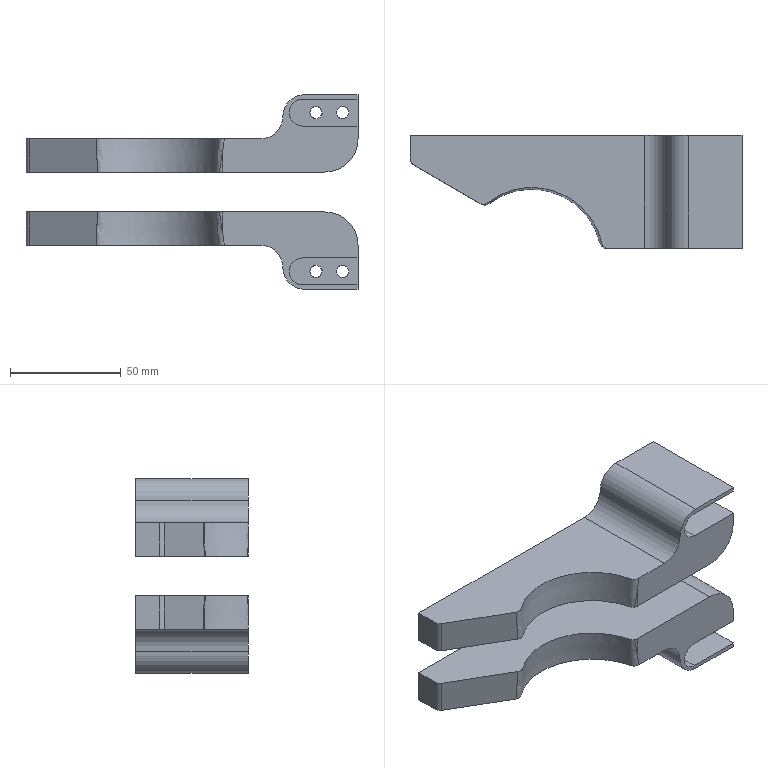NC program | NX | posted with a generic post | part box 150 x 51 x 88 mm
Lines 9175 to 9990 of 21241:
(FIXED_CONTOUR , TOOL : R4)
N18306 T08 M6
N18308 G54
N18310 G17 G0 G90 X12.055 Y-18.193 S9500 M3
N18312 G43 Z30. H8
N18314 Z4.4
N18316 G94 G1 Z0.185 F3000.
N18318 Y-18.066 Z0.019
N18320 Y-17.9 Z-0.108
N18322 Y-17.707 Z-0.188
N18324 Y-17.5 Z-0.215
N18326 X12.054 Y-13.737 Z-0.213
N18328 X12.065 Y-11.855 Z-0.236
N18330 X12.08 Y-9.973 Z-0.27
N18332 X12.09 Y-9.033 Z-0.29
N18334 X12.106 Y-8.383 Z-0.302
N18336 X12.156 Y-7.908 Z-0.298
N18338 X12.376 Y-6.012 Z-0.279
N18340 X12.618 Y-4.124 Z-0.251
N18342 X12.746 Y-3.183 Z-0.234
N18344 X12.88 Y-2.245 Z-0.219
N18346 X12.781 Y-2.244 Z-0.244
N18348 X12.649 Y-3.183 Z-0.261
N18350 X12.522 Y-4.124 Z-0.279
N18352 X12.28 Y-6.011 Z-0.308
N18354 X12.061 Y-7.907 Z-0.329
N18356 X12.011 Y-8.383 Z-0.333
N18358 X11.995 Y-9.033 Z-0.321
N18360 X11.985 Y-9.973 Z-0.301
N18362 X11.957 Y-13.737 Z-0.239
N18364 X11.958 Y-17.5 Z-0.24
N18366 X11.861 Z-0.267
N18368 Y-13.737
N18370 X11.89 Y-9.974 Z-0.332
N18372 X11.9 Y-9.033 Z-0.353
N18374 X11.917 Y-8.383 Z-0.365
N18376 X11.967 Y-7.907 Z-0.361
N18378 X12.185 Y-6.011 Z-0.339
N18380 X12.425 Y-4.123 Z-0.308
N18382 X12.552 Y-3.182 Z-0.289
N18384 X12.684 Y-2.243 Z-0.271
N18386 X12.587 Z-0.299
N18388 X12.456 Y-3.182 Z-0.318
N18390 X12.329 Y-4.123 Z-0.338
N18392 X12.09 Y-6.011 Z-0.371
N18394 X11.873 Y-7.907 Z-0.395
N18396 X11.823 Y-8.383 Z-0.399
N18398 X11.806 Y-9.033 Z-0.387
N18400 X11.796 Y-9.974 Z-0.365
N18402 X11.766 Y-13.737 Z-0.297
N18404 X11.765 Y-17.5 Z-0.295
N18406 X11.669 Z-0.325
N18408 X11.671 Y-13.737 Z-0.33
N18410 X11.703 Y-9.974 Z-0.399
N18412 X11.713 Y-9.033 Z-0.422
N18414 X11.73 Y-8.383 Z-0.434
N18416 X11.78 Y-7.907 Z-0.429
N18418 X11.996 Y-6.011 Z-0.405
N18420 X12.234 Y-4.122 Z-0.37
N18422 X12.36 Y-3.181 Z-0.349
N18424 X12.491 Y-2.242 Z-0.329
N18426 X12.395 Z-0.36
N18428 X12.265 Y-3.181 Z-0.381
N18430 X12.14 Y-4.122 Z-0.403
N18432 X11.902 Y-6.01 Z-0.439
N18434 X11.687 Y-7.907 Z-0.465
N18436 X11.638 Y-8.383 Z-0.471
N18438 X11.62 Y-9.033 Z-0.458
N18440 X11.61 Y-9.974 Z-0.435
N18442 X11.578 Y-13.737 Z-0.365
N18444 X11.574 Y-17.5 Z-0.355
N18446 X11.479 Z-0.387
N18448 X11.485 Y-13.737 Z-0.399
N18450 X11.518 Y-9.974 Z-0.471
N18452 X11.528 Y-9.033 Z-0.495
N18454 X11.546 Y-8.383 Z-0.508
N18456 X11.595 Y-7.907 Z-0.503
N18458 X11.809 Y-6.01 Z-0.475
N18460 X12.046 Y-4.122 Z-0.437
N18462 X12.17 Y-3.181 Z-0.414
N18464 X12.3 Y-2.241 Z-0.392
N18466 X12.205 Z-0.425
N18468 X12.076 Y-3.18 Z-0.449
N18470 X11.952 Y-4.122 Z-0.473
N18472 X11.717 Y-6.01 Z-0.513
N18474 X11.503 Y-7.907 Z-0.541
N18476 X11.454 Y-8.383 Z-0.547
N18478 X11.437 Y-9.033 Z-0.534
N18480 X11.426 Y-9.974 Z-0.509
N18482 X11.392 Y-13.737 Z-0.435
N18484 X11.386 Y-17.5 Z-0.421
N18486 X11.292 Z-0.455
N18488 Y-15.618
N18490 X11.3 Y-13.737 Z-0.471
N18492 X11.335 Y-9.974 Z-0.549
N18494 X11.346 Y-9.033 Z-0.574
N18496 X11.364 Y-8.383 Z-0.587
N18498 X11.412 Y-7.907 Z-0.581
N18500 X11.625 Y-6.01 Z-0.551
N18502 X11.859 Y-4.122 Z-0.51
N18504 X11.983 Y-3.18 Z-0.484
N18506 X12.111 Y-2.241 Z-0.46
N18508 X12.017 Z-0.496
N18510 X11.89 Y-3.18 Z-0.522
N18512 X11.767 Y-4.122 Z-0.548
N18514 X11.534 Y-6.011 Z-0.591
N18516 X11.322 Y-7.907 Z-0.622
N18518 X11.273 Y-8.383 Z-0.629
N18520 X11.256 Y-9.033 Z-0.615
N18522 X11.244 Y-9.974 Z-0.589
N18524 X11.208 Y-13.737 Z-0.51
N18526 X11.199 Y-15.618 Z-0.491
N18528 X11.2 Y-17.5
N18530 X11.107 Z-0.528
N18532 Y-15.618
N18534 X11.117 Y-13.737 Z-0.549
N18536 X11.154 Y-9.974 Z-0.631
N18538 X11.166 Y-9.033 Z-0.657
N18540 X11.184 Y-8.383 Z-0.671
N18542 X11.232 Y-7.908 Z-0.665
N18544 X11.443 Y-6.011 Z-0.632
N18546 X11.676 Y-4.122 Z-0.587
N18548 X11.798 Y-3.181 Z-0.56
N18550 X11.925 Y-2.241 Z-0.533
N18552 X11.832 Z-0.572
N18554 X11.706 Y-3.181 Z-0.6
N18556 X11.585 Y-4.122 Z-0.628
N18558 X11.353 Y-6.011 Z-0.674
N18560 X11.143 Y-7.908 Z-0.709
N18562 X11.095 Y-8.384 Z-0.715
N18564 X11.077 Y-9.033 Z-0.701
N18566 X11.065 Y-9.974 Z-0.674
N18568 X11.026 Y-13.737 Z-0.59
N18570 X11.016 Y-15.618 Z-0.568
N18572 Y-17.5 Z-0.567
N18574 X10.925 Z-0.607
N18576 X10.926 Y-15.618 Z-0.61
N18578 X10.937 Y-13.737 Z-0.632
N18580 X10.976 Y-9.974 Z-0.719
N18582 X10.988 Y-9.033 Z-0.746
N18584 X11.006 Y-8.384 Z-0.761
N18586 X11.054 Y-7.909 Z-0.754
N18588 X11.264 Y-6.012 Z-0.718
N18590 X11.494 Y-4.123 Z-0.67
N18592 X11.615 Y-3.181 Z-0.641
N18594 X11.741 Y-2.241 Z-0.612
N18596 X11.65 Y-2.242 Z-0.653
N18598 X11.525 Y-3.181 Z-0.683
N18600 X11.404 Y-4.123 Z-0.713
N18602 X11.175 Y-6.012 Z-0.763
N18604 X10.966 Y-7.909 Z-0.8
N18606 X10.918 Y-8.385 Z-0.807
N18608 X10.9 Y-9.033 Z-0.792
N18610 X10.888 Y-9.974 Z-0.764
N18612 X10.847 Y-13.737 Z-0.675
N18614 X10.837 Y-15.618 Z-0.652
N18616 X10.835 Y-17.5 Z-0.648
N18618 X10.745 Z-0.69
N18620 X10.747 Y-15.618 Z-0.695
N18622 X10.758 Y-13.737 Z-0.72
N18624 X10.8 Y-9.974 Z-0.811
N18626 X10.813 Y-9.033 Z-0.84
N18628 X10.831 Y-8.385 Z-0.855
N18630 X10.879 Y-7.91 Z-0.848
N18632 X11.086 Y-6.013 Z-0.809
N18634 X11.315 Y-4.124 Z-0.758
N18636 X11.559 Y-2.242 Z-0.696
N18638 X11.469 Z-0.74
N18640 X11.226 Y-4.124 Z-0.804
N18642 X10.999 Y-6.013 Z-0.857
N18644 X10.792 Y-7.91 Z-0.896
N18646 X10.744 Y-8.386 Z-0.904
N18648 X10.726 Y-9.033 Z-0.889
N18650 X10.713 Y-9.974 Z-0.859
N18652 X10.67 Y-13.737 Z-0.766
N18654 X10.659 Y-15.618 Z-0.74
N18656 X10.656 Y-17.5 Z-0.734
N18658 X10.567 Z-0.779
N18660 X10.57 Y-15.618 Z-0.786
N18662 X10.583 Y-13.737 Z-0.813
N18664 X10.626 Y-9.974 Z-0.909
N18666 X10.64 Y-9.033 Z-0.939
N18668 X10.658 Y-8.386 Z-0.955
N18670 X10.706 Y-7.911 Z-0.947
N18672 X10.912 Y-6.014 Z-0.906
N18674 X11.138 Y-4.125 Z-0.851
N18676 X11.38 Y-2.243 Z-0.785
N18678 X11.291 Y-2.244 Z-0.832
N18680 X11.051 Y-4.125 Z-0.9
N18682 X10.825 Y-6.015 Z-0.956
N18684 X10.62 Y-7.912 Z-0.998
N18686 X10.573 Y-8.387 Z-1.006
N18688 X10.554 Y-9.033 Z-0.99
N18690 X10.54 Y-9.974 Z-0.96
N18692 X10.496 Y-13.737 Z-0.861
N18694 X10.483 Y-15.618 Z-0.833
N18696 X10.479 Y-17.5 Z-0.825
N18698 X10.392 Z-0.872
N18700 X10.396 Y-15.618 Z-0.882
N18702 X10.409 Y-13.737 Z-0.911
N18704 X10.455 Y-9.974 Z-1.012
N18706 X10.469 Y-9.033 Z-1.043
N18708 X10.488 Y-8.388 Z-1.06
N18710 X10.535 Y-7.912 Z-1.051
N18712 X10.739 Y-6.016 Z-1.007
N18714 X10.964 Y-4.126 Z-0.949
N18716 X11.203 Y-2.244 Z-0.879
N18718 X11.116 Y-2.245 Z-0.928
N18720 X10.877 Y-4.127 Z-1.
N18722 X10.654 Y-6.016 Z-1.06
N18724 X10.45 Y-7.913 Z-1.105
N18726 X10.404 Y-8.389 Z-1.114
N18728 X10.385 Y-9.033 Z-1.097
N18730 X10.37 Y-9.974 Z-1.065
N18732 X10.323 Y-13.737 Z-0.962
N18734 X10.31 Y-15.618 Z-0.932
N18736 X10.305 Y-17.5 Z-0.921
N18738 X10.218 Z-0.971
N18740 X10.224 Y-15.619 Z-0.983
N18742 X10.238 Y-13.737 Z-1.015
N18744 X10.286 Y-9.974 Z-1.12
N18746 X10.301 Y-9.033 Z-1.153
N18748 X10.32 Y-8.39 Z-1.17
N18750 X10.367 Y-7.914 Z-1.16
N18752 X10.569 Y-6.017 Z-1.114
N18754 X10.791 Y-4.128 Z-1.053
N18756 X11.029 Y-2.246 Z-0.979
N18758 X10.942 Y-2.247 Z-1.031
N18760 X10.706 Y-4.129 Z-1.107
N18762 X10.485 Y-6.018 Z-1.169
N18764 X10.283 Y-7.915 Z-1.217
N18766 X10.237 Y-8.391 Z-1.227
N18768 X10.218 Y-9.033 Z-1.209
N18770 X10.203 Y-9.974 Z-1.176
N18772 X10.154 Y-13.737 Z-1.068
N18774 X10.139 Y-15.619 Z-1.036
N18776 X10.133 Y-17.5 Z-1.023
N18778 X10.048 Z-1.075
N18780 X10.054 Y-15.619 Z-1.089
N18782 X10.07 Y-13.737 Z-1.123
N18784 X10.12 Y-9.974 Z-1.234
N18786 X10.135 Y-9.033 Z-1.267
N18788 X10.154 Y-8.392 Z-1.285
N18790 X10.201 Y-7.916 Z-1.275
N18792 X10.401 Y-6.02 Z-1.226
N18794 X10.622 Y-4.13 Z-1.162
N18796 X10.856 Y-2.248 Z-1.084
N18798 X10.771 Y-2.249 Z-1.138
N18800 X10.538 Y-4.132 Z-1.218
N18802 X10.318 Y-6.021 Z-1.284
N18804 X10.119 Y-7.917 Z-1.335
N18806 X10.072 Y-8.393 Z-1.345
N18808 X10.053 Y-9.033 Z-1.327
N18810 X10.038 Y-9.974 Z-1.293
N18812 X9.986 Y-13.737 Z-1.18
N18814 X9.97 Y-15.619 Z-1.145
N18816 X9.963 Y-17.5 Z-1.129
N18818 X9.879 Z-1.184
N18820 X9.887 Y-15.619 Z-1.201
N18822 X9.903 Y-13.737 Z-1.237
N18824 X9.956 Y-9.974 Z-1.353
N18826 X9.972 Y-9.033 Z-1.388
N18828 X9.991 Y-8.394 Z-1.406
N18830 X10.037 Y-7.919 Z-1.395
N18832 X10.236 Y-6.022 Z-1.344
N18834 X10.454 Y-4.133 Z-1.276
N18836 X10.687 Y-2.25 Z-1.194
N18838 X10.603 Y-2.252 Z-1.251
N18840 X10.372 Y-4.134 Z-1.335
N18842 X10.154 Y-6.023 Z-1.405
N18844 X9.956 Y-7.92 Z-1.458
N18846 X9.91 Y-8.395 Z-1.468
N18848 X9.891 Y-9.033 Z-1.45
N18850 X9.875 Y-9.974 Z-1.414
N18852 X9.821 Y-13.737 Z-1.296
N18854 X9.804 Y-15.619 Z-1.259
N18856 X9.796 Y-17.5 Z-1.241
N18858 X9.713 Z-1.299
N18860 X9.722 Y-15.619 Z-1.318
N18862 X9.74 Y-13.737 Z-1.357
N18864 X9.794 Y-9.974 Z-1.477
N18866 X9.811 Y-9.033 Z-1.513
N18868 X9.83 Y-8.396 Z-1.532
N18870 X9.876 Y-7.921 Z-1.521
N18872 X10.073 Y-6.025 Z-1.467
N18874 X10.29 Y-4.136 Z-1.396
N18876 X10.519 Y-2.253 Z-1.31
N18878 X10.437 Y-2.255 Z-1.369
N18880 X10.208 Y-4.137 Z-1.458
N18882 X9.993 Y-6.026 Z-1.53
N18884 X9.796 Y-7.923 Z-1.586
N18886 X9.751 Y-8.398 Z-1.597
N18888 X9.731 Y-9.033 Z-1.578
N18890 X9.715 Y-9.974 Z-1.542
N18892 X9.659 Y-13.737 Z-1.418
N18894 X9.64 Y-15.619 Z-1.379
N18896 X9.631 Y-17.5 Z-1.359
N18898 X9.55 Z-1.419
N18900 X9.56 Y-15.619 Z-1.44
N18902 X9.578 Y-13.737 Z-1.482
N18904 X9.635 Y-9.974 Z-1.607
N18906 X9.653 Y-9.034 Z-1.645
N18908 X9.672 Y-8.399 Z-1.664
N18910 X9.718 Y-7.924 Z-1.653
N18912 X9.913 Y-6.028 Z-1.595
N18914 X10.127 Y-4.139 Z-1.521
N18916 X10.355 Y-2.256 Z-1.431
N18918 X10.273 Y-2.258 Z-1.493
N18920 X10.047 Y-4.14 Z-1.586
N18922 X9.834 Y-6.03 Z-1.662
N18924 X9.639 Y-7.926 Z-1.72
N18926 X9.594 Y-8.401 Z-1.732
N18928 X9.574 Y-9.034 Z-1.713
N18930 X9.557 Y-9.974 Z-1.675
N18932 X9.499 Y-13.737 Z-1.546
N18934 X9.479 Y-15.619 Z-1.504
N18936 X9.469 Y-17.5 Z-1.481
N18938 X9.389 Z-1.545
N18940 X9.4 Y-15.619 Z-1.568
N18942 X9.42 Y-13.737 Z-1.612
N18944 X9.479 Y-9.974 Z-1.743
N18946 X9.497 Y-9.034 Z-1.782
N18948 X9.517 Y-8.402 Z-1.802
N18950 X9.562 Y-7.927 Z-1.79
N18952 X9.755 Y-6.031 Z-1.73
N18954 X9.967 Y-4.142 Z-1.652
N18956 X10.192 Y-2.26 Z-1.557
N18958 X10.112 Y-2.261 Z-1.623
N18960 X9.889 Y-4.144 Z-1.719
N18962 X9.678 Y-6.033 Z-1.799
N18964 X9.485 Y-7.929 Z-1.86
N18966 X9.44 Y-8.404 Z-1.873
N18968 X9.42 Y-9.034 Z-1.853
N18970 X9.402 Y-9.974 Z-1.813
N18972 X9.341 Y-13.737 Z-1.679
N18974 X9.321 Y-15.619 Z-1.635
N18976 X9.31 Y-17.5 Z-1.61
N18978 X9.231 Z-1.676
N18980 X9.242 Y-15.619 Z-1.702
N18982 X9.263 Y-13.737 Z-1.748
N18984 X9.326 Y-9.974 Z-1.885
N18986 X9.344 Y-9.034 Z-1.925
N18988 X9.364 Y-8.406 Z-1.945
N18990 X9.409 Y-7.931 Z-1.933
N18992 X9.6 Y-6.035 Z-1.87
N18994 X9.81 Y-4.146 Z-1.788
N18996 X10.033 Y-2.263 Z-1.69
N18998 X9.954 Y-2.265 Z-1.758
N19000 X9.733 Y-4.148 Z-1.859
N19002 X9.524 Y-6.037 Z-1.942
N19004 X9.333 Y-7.932 Z-2.007
N19006 X9.289 Y-8.407 Z-2.02
N19008 X9.268 Y-9.034 Z-1.999
N19010 X9.25 Y-9.974 Z-1.958
N19012 X9.186 Y-13.737 Z-1.819
N19014 X9.165 Y-15.619 Z-1.771
N19016 X9.152 Y-17.5 Z-1.744
N19018 X9.075 Z-1.813
N19020 X9.088 Y-15.619 Z-1.842
N19022 X9.11 Y-13.737 Z-1.89
N19024 X9.175 Y-9.974 Z-2.033
N19026 X9.194 Y-9.034 Z-2.074
N19028 X9.214 Y-8.409 Z-2.095
N19030 X9.258 Y-7.934 Z-2.082
N19032 X9.448 Y-6.039 Z-2.016
N19034 X9.656 Y-4.15 Z-1.931
N19036 X9.876 Y-2.268 Z-1.828
N19038 X9.798 Y-2.27 Z-1.9
N19040 X9.58 Y-4.153 Z-2.005
N19042 X9.373 Y-6.041 Z-2.092
N19044 X9.184 Y-7.936 Z-2.159
N19046 X9.14 Y-8.411 Z-2.172
N19048 X9.12 Y-9.034 Z-2.151
N19050 X9.1 Y-9.974 Z-2.109
N19052 X9.034 Y-13.737 Z-1.964
N19054 X9.011 Y-15.619 Z-1.914
N19056 X8.998 Y-17.5 Z-1.884
N19058 X8.922 Z-1.956
N19060 X8.936 Y-15.619 Z-1.987
N19062 X8.959 Y-13.737 Z-2.039
N19064 X9.027 Y-9.974 Z-2.187
N19066 X9.046 Y-9.034 Z-2.23
N19068 X9.067 Y-8.413 Z-2.251
N19070 X9.111 Y-7.938 Z-2.237
N19072 X9.299 Y-6.043 Z-2.169
N19074 X9.504 Y-4.155 Z-2.08
N19076 X9.721 Y-2.272 Z-1.973
N19078 X9.645 Y-2.275 Z-2.047
N19080 X9.429 Y-4.157 Z-2.157
N19082 X9.225 Y-6.046 Z-2.247
N19084 X9.038 Y-7.94 Z-2.318
N19086 X8.994 Y-8.415 Z-2.332
N19088 X8.974 Y-9.034 Z-2.31
N19090 X8.954 Y-9.974 Z-2.266
N19092 X8.885 Y-13.737 Z-2.115
N19094 X8.861 Y-15.619 Z-2.062
N19096 X8.846 Y-17.5 Z-2.03
N19098 X8.772 Z-2.105
N19100 X8.787 Y-15.619 Z-2.139
N19102 X8.812 Y-13.737 Z-2.193
N19104 X8.882 Y-9.974 Z-2.347
N19106 X8.902 Y-9.034 Z-2.392
N19108 X8.923 Y-8.417 Z-2.414
N19110 X8.966 Y-7.942 Z-2.399
N19112 X9.152 Y-6.048 Z-2.328
N19114 X9.355 Y-4.16 Z-2.235
N19116 X9.57 Y-2.277 Z-2.123
N19118 X9.495 Y-2.28 Z-2.201
N19120 X9.282 Y-4.162 Z-2.315
N19122 X9.08 Y-6.051 Z-2.41
N19124 X8.895 Y-7.945 Z-2.483
N19126 X8.852 Y-8.419 Z-2.498
N19128 X8.831 Y-9.034 Z-2.476
N19130 X8.81 Y-9.975 Z-2.43
N19132 X8.739 Y-13.737 Z-2.273
N19134 X8.713 Y-15.619 Z-2.217
N19136 X8.697 Y-17.5 Z-2.182
N19138 X8.624 Z-2.261
N19140 X8.641 Y-15.619 Z-2.297
N19142 X8.667 Y-13.737 Z-2.354
N19144 X8.74 Y-9.975 Z-2.515
N19146 X8.761 Y-9.034 Z-2.561
N19148 X8.782 Y-8.422 Z-2.583
N19150 X8.825 Y-7.947 Z-2.568
N19152 X9.009 Y-6.053 Z-2.493
N19154 X9.209 Y-4.165 Z-2.397
N19156 X9.421 Y-2.282 Z-2.28
N19158 X9.348 Y-2.285 Z-2.362
N19160 X9.138 Y-4.168 Z-2.48
N19162 X8.938 Y-6.056 Z-2.579
N19164 X8.755 Y-7.949 Z-2.655
N19166 X8.712 Y-8.424 Z-2.671
N19168 X8.691 Y-9.034 Z-2.648
N19170 X8.67 Y-9.975 Z-2.601
N19172 X8.595 Y-13.737 Z-2.437
N19174 X8.569 Y-15.619 Z-2.378
N19176 X8.552 Y-17.5 Z-2.341
N19178 X8.48 Z-2.423
N19180 X8.497 Y-15.619 Z-2.462
N19182 X8.525 Y-13.737 Z-2.522
N19184 X8.601 Y-9.975 Z-2.689
N19186 X8.623 Y-9.034 Z-2.737
N19188 X8.644 Y-8.426 Z-2.76
N19190 X8.686 Y-7.952 Z-2.744
N19192 X8.868 Y-6.059 Z-2.666
N19194 X9.067 Y-4.171 Z-2.565
N19196 X9.276 Y-2.288 Z-2.444
N19198 X9.204 Y-2.291 Z-2.529
N19200 X8.996 Y-4.174 Z-2.652
N19202 X8.8 Y-6.061 Z-2.755
N19204 X8.619 Y-7.955 Z-2.835
N19206 X8.576 Y-8.429 Z-2.851
N19208 X8.555 Y-9.034 Z-2.828
N19210 X8.533 Y-9.975 Z-2.779
N19212 X8.455 Y-13.737 Z-2.609
N19214 X8.427 Y-15.619 Z-2.547
N19216 X8.409 Y-17.5 Z-2.506
N19218 X8.338 Z-2.591
N19220 X8.357 Y-15.619 Z-2.633
N19222 X8.386 Y-13.737 Z-2.697
N19224 X8.465 Y-9.975 Z-2.871
N19226 X8.488 Y-9.034 Z-2.921
N19228 X8.51 Y-8.431 Z-2.944
N19230 X8.552 Y-7.957 Z-2.928
N19232 X8.732 Y-6.064 Z-2.846
N19234 X8.927 Y-4.177 Z-2.741
N19236 X9.133 Y-2.294 Z-2.615
N19238 X9.063 Y-2.298 Z-2.703
N19240 X8.859 Y-4.18 Z-2.832
N19242 X8.664 Y-6.067 Z-2.939
N19244 X8.486 Y-7.96 Z-3.022
N19246 X8.444 Y-8.434 Z-3.039
N19248 X8.422 Y-9.034 Z-3.016
N19250 X8.399 Y-9.975 Z-2.965
N19252 X8.318 Y-13.737 Z-2.787
N19254 X8.289 Y-15.619 Z-2.722
N19256 X8.269 Y-17.5 Z-2.678
N19258 X8.2 Z-2.767
N19260 X8.221 Y-15.619 Z-2.812
N19262 X8.251 Y-13.737 Z-2.88
N19264 X8.334 Y-9.975 Z-3.061
N19266 X8.357 Y-9.034 Z-3.113
N19268 X8.379 Y-8.437 Z-3.137
N19270 X8.42 Y-7.963 Z-3.119
N19272 X8.598 Y-6.071 Z-3.033
N19274 X8.791 Y-4.183 Z-2.924
N19276 X8.994 Y-2.301 Z-2.793
N19278 X8.926 Y-2.304 Z-2.885
N19280 X8.724 Y-4.187 Z-3.019
N19282 X8.533 Y-6.074 Z-3.13
N19284 X8.356 Y-7.966 Z-3.218
N19286 X8.315 Y-8.44 Z-3.236
N19288 X8.293 Y-9.034 Z-3.212
N19290 X8.269 Y-9.975 Z-3.159
N19292 X8.185 Y-13.737 Z-2.974
N19294 X8.154 Y-15.619 Z-2.905
N19296 X8.133 Y-17.5 Z-2.858
N19298 X8.066 Z-2.951
N19300 X8.088 Y-15.619 Z-2.999
N19302 X8.12 Y-13.737 Z-3.07
N19304 X8.206 Y-9.975 Z-3.259
N19306 X8.23 Y-9.034 Z-3.313
N19308 X8.252 Y-8.443 Z-3.337
N19310 X8.293 Y-7.969 Z-3.319
N19312 X8.468 Y-6.077 Z-3.229
N19314 X8.658 Y-4.19 Z-3.115
N19316 X8.859 Y-2.308 Z-2.979
N19318 X8.792 Y-2.312 Z-3.075
N19320 X8.594 Y-4.194 Z-3.214
N19322 X8.405 Y-6.081 Z-3.331
N19324 X8.231 Y-7.972 Z-3.422
N19326 X8.19 Y-8.446 Z-3.441
N19328 X8.168 Y-9.034 Z-3.416
N19330 X8.143 Y-9.975 Z-3.361
N19332 X8.055 Y-13.737 Z-3.168
N19334 X8.022 Y-15.619 Z-3.096
N19336 X8. Y-17.5 Z-3.046
N19338 X7.935 Z-3.142
N19340 X7.958 Y-15.619 Z-3.194
N19342 X7.992 Y-13.737 Z-3.269
N19344 X8.082 Y-9.975 Z-3.466
N19346 X8.107 Y-9.034 Z-3.522
N19348 X8.129 Y-8.449 Z-3.547
N19350 X8.17 Y-7.975 Z-3.528
N19352 X8.343 Y-6.084 Z-3.434
N19354 X8.53 Y-4.198 Z-3.315
N19356 X8.727 Y-2.316 Z-3.173
N19358 X8.662 Y-2.32 Z-3.273
N19360 X8.467 Y-4.202 Z-3.418
N19362 X8.281 Y-6.088 Z-3.54
N19364 X8.11 Y-7.979 Z-3.636
N19366 X8.07 Y-8.452 Z-3.655
N19368 X8.047 Y-9.034 Z-3.63
N19370 X8.021 Y-9.975 Z-3.573
N19372 X7.93 Y-13.737 Z-3.371
N19374 X7.895 Y-15.619 Z-3.295
N19376 X7.871 Y-17.5 Z-3.241
N19378 X7.807 Z-3.342
N19380 X7.833 Y-15.619 Z-3.398
N19382 X7.868 Y-13.737 Z-3.476
N19384 X7.962 Y-9.975 Z-3.682
N19386 X7.989 Y-9.034 Z-3.741
N19388 X8.011 Y-8.455 Z-3.766
N19390 X8.051 Y-7.982 Z-3.746
N19392 X8.221 Y-6.092 Z-3.648
N19394 X8.405 Y-4.206 Z-3.524
N19396 X8.599 Y-2.324 Z-3.376
N19398 X8.536 Y-2.328 Z-3.481
N19400 X8.344 Y-4.21 Z-3.632
N19402 X8.162 Y-6.096 Z-3.759
N19404 X7.993 Y-7.986 Z-3.859
N19406 X7.954 Y-8.459 Z-3.88
N19408 X7.931 Y-9.034 Z-3.854
N19410 X7.904 Y-9.975 Z-3.794
N19412 X7.808 Y-13.737 Z-3.584
N19414 X7.771 Y-15.619 Z-3.503
N19416 X7.745 Y-17.5 Z-3.445
N19418 X7.715 Z-3.498
N19420 X7.684 Z-3.551
N19422 X7.711 Y-15.619 Z-3.61
N19424 X7.749 Y-13.737 Z-3.693
N19426 X7.847 Y-9.975 Z-3.909
N19428 X7.875 Y-9.034 Z-3.97
N19430 X7.898 Y-8.463 Z-3.996
N19432 X7.937 Y-7.99 Z-3.975
N19434 X8.104 Y-6.1 Z-3.872
N19436 X8.285 Y-4.214 Z-3.742
N19438 X8.475 Y-2.332 Z-3.588
N19440 X8.445 Y-2.335 Z-3.643
N19442 X8.415 Y-2.337 Z-3.698
N19444 X8.227 Y-4.219 Z-3.855
N19446 X8.047 Y-6.104 Z-3.988
N19448 X7.882 Y-7.993 Z-4.094
N19450 X7.843 Y-8.466 Z-4.116
N19452 X7.82 Y-9.034 Z-4.089
N19454 X7.791 Y-9.975 Z-4.027
N19456 X7.691 Y-13.737 Z-3.806
N19458 X7.652 Y-15.619 Z-3.721
N19460 X7.624 Y-17.5 Z-3.659
N19462 X7.595 Z-3.714
N19464 X7.566 Z-3.77
N19466 X7.595 Y-15.619 Z-3.833
N19468 X7.634 Y-13.737 Z-3.921
N19470 X7.737 Y-9.975 Z-4.147
N19472 X7.766 Y-9.034 Z-4.211
N19474 X7.789 Y-8.47 Z-4.238
N19476 X7.828 Y-7.997 Z-4.216
N19478 X7.992 Y-6.109 Z-4.107
N19480 X8.169 Y-4.224 Z-3.971
N19482 X8.355 Y-2.342 Z-3.81
N19484 X8.326 Y-2.344 Z-3.867
N19486 X8.298 Y-2.346 Z-3.925
N19488 X8.114 Y-4.228 Z-4.09
N19490 X7.938 Y-6.113 Z-4.229
N19492 X7.775 Y-8.001 Z-4.341
N19494 X7.737 Y-8.474 Z-4.363
N19496 X7.714 Y-9.034 Z-4.336
N19498 X7.684 Y-9.975 Z-4.271
N19500 X7.579 Y-13.738 Z-4.039
N19502 X7.538 Y-15.619 Z-3.949
N19504 X7.521 Y-16.559 Z-3.912
N19506 X7.508 Y-17.5 Z-3.883
N19508 X7.48 Z-3.94
N19510 X7.452 Z-3.999
N19512 X7.465 Y-16.559 Z-4.029
N19514 X7.483 Y-15.619 Z-4.067
N19516 X7.525 Y-13.738 Z-4.16
N19518 X7.633 Y-9.975 Z-4.397
N19520 X7.663 Y-9.034 Z-4.464
N19522 X7.687 Y-8.478 Z-4.492
N19524 X7.725 Y-8.006 Z-4.469
N19526 X7.886 Y-6.118 Z-4.355
N19528 X8.059 Y-4.233 Z-4.211
N19530 X8.241 Y-2.351 Z-4.043
N19532 X8.213 Y-2.354 Z-4.103
N19534 X8.186 Y-2.357 Z-4.164
N19536 X8.006 Y-4.238 Z-4.336
N19538 X7.835 Y-6.123 Z-4.483
N19540 X7.675 Y-8.01 Z-4.6
N19542 X7.638 Y-8.483 Z-4.625
N19544 X7.614 Y-9.034 Z-4.597
N19546 X7.583 Y-9.975 Z-4.528
N19548 X7.472 Y-13.738 Z-4.284
N19550 X7.429 Y-15.619 Z-4.188
N19552 X7.411 Y-16.559 Z-4.149
N19554 X7.397 Y-17.5 Z-4.117
N19556 X7.37 Z-4.178
N19558 X7.343 Z-4.239
N19560 X7.358 Y-16.559 Z-4.272
N19562 X7.376 Y-15.619 Z-4.313
N19564 X7.421 Y-13.738 Z-4.411
N19566 X7.535 Y-9.975 Z-4.662
N19568 X7.567 Y-9.034 Z-4.732
N19570 X7.591 Y-8.487 Z-4.761
N19572 X7.628 Y-8.015 Z-4.736
N19574 X7.785 Y-6.128 Z-4.615
N19576 X7.954 Y-4.244 Z-4.464
N19578 X8.132 Y-2.362 Z-4.288
N19580 X8.105 Y-2.365 Z-4.351
N19582 X8.079 Y-2.368 Z-4.415
N19584 X7.904 Y-4.249 Z-4.596
N19586 X7.737 Y-6.133 Z-4.751
N19588 X7.582 Y-8.02 Z-4.875
N19590 X7.545 Y-8.492 Z-4.901
N19592 X7.522 Y-9.035 Z-4.872
N19594 X7.489 Y-9.975 Z-4.8
N19596 X7.372 Y-13.738 Z-4.542
N19598 X7.325 Y-15.619 Z-4.44
N19600 X7.306 Y-16.559 Z-4.398
N19602 X7.291 Y-17.5 Z-4.364
N19604 X7.265 Z-4.428
N19606 X7.24 Z-4.492
N19608 X7.256 Y-16.559 Z-4.528
N19610 X7.276 Y-15.619 Z-4.571
N19612 X7.324 Y-13.738 Z-4.677
N19614 X7.444 Y-9.975 Z-4.942
N19616 X7.478 Y-9.035 Z-5.017
N19618 X7.502 Y-8.496 Z-5.046
N19620 X7.538 Y-8.025 Z-5.019
N19622 X7.692 Y-6.139 Z-4.891
N19624 X7.856 Y-4.255 Z-4.731
N19626 X8.029 Y-2.374 Z-4.545
N19628 X8.004 Y-2.377 Z-4.612
N19630 X7.979 Y-2.38 Z-4.68
N19632 X7.81 Y-4.261 Z-4.871
N19634 X7.648 Y-6.144 Z-5.035
N19636 X7.497 Y-8.03 Z-5.168
N19638 X7.461 Y-8.502 Z-5.195
N19640 X7.437 Y-9.035 Z-5.166
N19642 X7.402 Y-9.975 Z-5.089
N19644 X7.278 Y-13.738 Z-4.815
N19646 X7.228 Y-15.619 Z-4.706
N19648 X7.208 Y-16.559 Z-4.661
N19650 X7.191 Y-17.5 Z-4.624
N19652 X7.167 Z-4.692
N19654 X7.144 Z-4.76
N19656 X7.161 Y-16.559 Z-4.798
N19658 X7.182 Y-15.619 Z-4.845
N19660 X7.234 Y-13.738 Z-4.958
N19662 X7.362 Y-9.975 Z-5.241
N19664 X7.398 Y-9.035 Z-5.32
N19666 X7.422 Y-8.507 Z-5.35
N19668 X7.458 Y-8.035 Z-5.322
N19670 X7.606 Y-6.15 Z-5.184
N19672 X7.765 Y-4.267 Z-5.015
N19674 X7.932 Y-2.386 Z-4.818
N19676 X7.909 Y-2.389 Z-4.889
N19678 X7.887 Y-2.392 Z-4.961
N19680 X7.723 Y-4.274 Z-5.163
N19682 X7.567 Y-6.157 Z-5.339
N19684 X7.42 Y-8.041 Z-5.479
N19686 X7.385 Y-8.512 Z-5.507
N19688 X7.361 Y-9.035 Z-5.477
N19690 X7.324 Y-9.975 Z-5.397
N19692 X7.192 Y-13.738 Z-5.105
N19694 X7.139 Y-15.619 Z-4.989
N19696 X7.116 Y-16.559 Z-4.939
N19698 X7.098 Y-17.5 Z-4.9
N19700 X7.076 Z-4.971
N19702 X7.055 Z-5.044
N19704 X7.073 Y-16.559 Z-5.085
N19706 X7.097 Y-15.619 Z-5.137
N19708 X7.152 Y-13.738 Z-5.258
N19710 X7.286 Y-9.975 Z-5.554
N19712 X7.323 Y-9.035 Z-5.634
N19714 X7.347 Y-8.517 Z-5.663
N19716 X7.382 Y-8.046 Z-5.635
N19718 X7.529 Y-6.163 Z-5.496
N19720 X7.683 Y-4.28 Z-5.317
N19722 X7.843 Y-2.399 Z-5.108
N19724 X7.822 Y-2.403 Z-5.183
N19726 X7.802 Y-2.406 Z-5.26
N19728 X7.645 Y-4.287 Z-5.475
N19730 X7.491 Y-6.169 Z-5.654
N19732 X7.343 Y-8.052 Z-5.79
N19734 X7.308 Y-8.523 Z-5.818
N19736 X7.284 Y-9.035 Z-5.789
N19738 X7.248 Y-9.975 Z-5.709
N19740 X7.114 Y-13.738 Z-5.414
N19742 X7.057 Y-15.619 Z-5.29
N19744 X7.033 Y-16.559 Z-5.236
N19746 X7.013 Y-17.5 Z-5.192
N19748 X6.993 Z-5.269
N19750 X6.974 Z-5.346
N19752 X6.995 Y-16.559 Z-5.392
N19754 X7.019 Y-15.619 Z-5.446
N19756 X7.076 Y-13.738 Z-5.571
N19758 X7.209 Y-9.975 Z-5.864
N19760 X7.245 Y-9.035 Z-5.943
N19762 X7.268 Y-8.528 Z-5.971
N19764 X7.304 Y-8.057 Z-5.944
N19766 X7.452 Y-6.176 Z-5.81
N19768 X7.607 Y-4.294 Z-5.633
N19770 X7.763 Y-2.414 Z-5.417
N19772 X7.744 Y-2.417 Z-5.497
N19774 X7.725 Y-2.421 Z-5.577
N19776 X7.568 Y-4.301 Z-5.79
N19778 X7.413 Y-6.182 Z-5.964
N19780 X7.264 Y-8.063 Z-6.097
N19782 X7.229 Y-8.533 Z-6.123
N19784 X7.205 Y-9.035 Z-6.095
N19786 X7.17 Y-9.975 Z-6.017
N19788 X7.037 Y-13.738 Z-5.725
N19790 X6.981 Y-15.619 Z-5.602
N19792 X6.957 Y-16.559 Z-5.548
N19794 X6.936 Y-17.5 Z-5.503
N19796 X6.917 Z-5.581
N19798 X6.898 Z-5.659
N19800 X6.918 Y-16.559 Z-5.704
N19802 X6.943 Y-15.619 Z-5.757
N19804 X6.998 Y-13.738 Z-5.879
N19806 X7.13 Y-9.975 Z-6.168
N19808 X7.165 Y-9.035 Z-6.247
N19810 X7.188 Y-8.538 Z-6.274
N19812 X7.224 Y-8.068 Z-6.248
N19814 X7.373 Y-6.188 Z-6.118
N19816 X7.529 Y-4.308 Z-5.946
N19818 X7.687 Y-2.429 Z-5.735
N19820 X7.668 Y-2.432 Z-5.814
N19822 X7.648 Y-2.436 Z-5.892
N19824 X7.49 Y-4.315 Z-6.1
N19826 X7.333 Y-6.194 Z-6.27
N19828 X7.183 Y-8.073 Z-6.398
N19830 X7.147 Y-8.543 Z-6.424
N19832 X7.124 Y-9.035 Z-6.397
N19834 X7.089 Y-9.975 Z-6.319
N19836 X6.958 Y-13.738 Z-6.031
N19838 X6.903 Y-15.619 Z-5.91
N19840 X6.879 Y-16.559 Z-5.858
N19842 X6.859 Y-17.5 Z-5.814
N19844 X6.84 Z-5.891
N19846 X6.82 Z-5.967
N19848 X6.84 Y-16.559 Z-6.01
N19850 X6.863 Y-15.619 Z-6.062
N19852 X6.918 Y-13.738 Z-6.182
N19854 X7.048 Y-9.975 Z-6.468
N19856 X7.083 Y-9.035 Z-6.546
N19858 X7.106 Y-8.548 Z-6.572
N19860 X7.142 Y-8.078 Z-6.547
N19862 X7.292 Y-6.2 Z-6.42
N19864 X7.449 Y-4.322 Z-6.253
N19866 X7.608 Y-2.443 Z-6.048
N19868 X7.588 Y-2.447 Z-6.125
N19870 X7.568 Y-2.45 Z-6.202
N19872 X7.408 Y-4.328 Z-6.405
N19874 X7.251 Y-6.206 Z-6.57
N19876 X7.1 Y-8.083 Z-6.695
N19878 X7.063 Y-8.553 Z-6.719
N19880 X7.041 Y-9.035 Z-6.693
N19882 X7.006 Y-9.975 Z-6.616
N19884 X6.877 Y-13.738 Z-6.332
N19886 X6.823 Y-15.619 Z-6.213
N19888 X6.8 Y-16.559 Z-6.162
N19890 X6.78 Y-17.5 Z-6.119
N19892 X6.76 Z-6.195
N19894 X6.74 Z-6.27
N19896 X6.759 Y-16.559 Z-6.312
N19898 X6.782 Y-15.619 Z-6.363
N19900 X6.835 Y-13.738 Z-6.48
N19902 X6.964 Y-9.975 Z-6.763
N19904 X6.999 Y-9.035 Z-6.84
N19906 X7.021 Y-8.557 Z-6.866
N19908 X7.057 Y-8.088 Z-6.841
N19910 X7.209 Y-6.211 Z-6.719
N19912 X7.367 Y-4.335 Z-6.556
N19914 X7.528 Y-2.457 Z-6.355
N19916 X7.507 Y-2.461 Z-6.431
N19918 X7.486 Y-2.464 Z-6.507
N19920 X7.325 Y-4.341 Z-6.705
N19922 X7.166 Y-6.217 Z-6.866
N19924 X7.014 Y-8.093 Z-6.987
N19926 X6.978 Y-8.562 Z-7.011
N19928 X6.956 Y-9.035 Z-6.986
N19930 X6.921 Y-9.975 Z-6.909